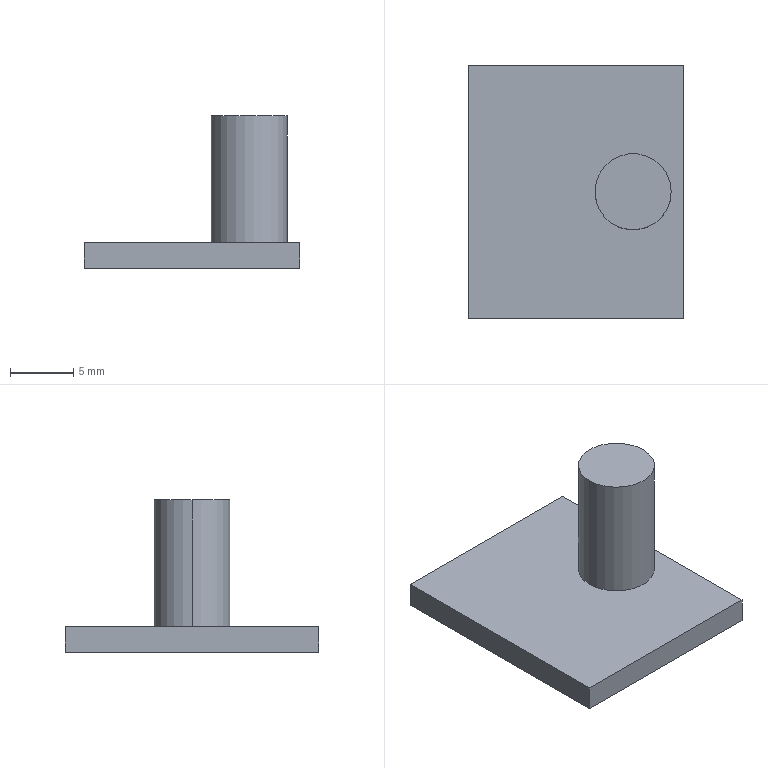Part | SolidWorks | features FlatPattern 1, ICE 1, SMBaseFlange 1, SheetMetal 1 | 1 solid | 9 faces | box 17 x 20 x 12 mm | volume 962.743 mm3 | plane 7 | cylinder 2 | commonest cylinder face diameters 6 x2
STEP:
#1=CARTESIAN_POINT('',(7.5,0.,10.));
#2=VERTEX_POINT('',#1);
#3=CARTESIAN_POINT('',(1.5,0.,10.));
#4=VERTEX_POINT('',#3);
#5=CARTESIAN_POINT('',(4.5,0.,10.));
#6=DIRECTION('',(0.,0.,1.));
#7=DIRECTION('',(1.,0.,0.));
#8=AXIS2_PLACEMENT_3D('',#5,#6,#7);
#9=CIRCLE('',#8,3.);
#10=EDGE_CURVE('',#2,#4,#9,.T.);
#11=ORIENTED_EDGE('',*,*,#10,.F.);
#12=CARTESIAN_POINT('',(7.5,0.,0.));
#13=VERTEX_POINT('',#12);
#14=CARTESIAN_POINT('',(7.5,0.,10.));
#15=DIRECTION('',(0.,0.,-1.));
#16=VECTOR('',#15,1000.);
#17=LINE('',#14,#16);
#18=EDGE_CURVE('',#2,#13,#17,.T.);
#19=ORIENTED_EDGE('',*,*,#18,.T.);
#20=CARTESIAN_POINT('',(1.5,0.,0.));
#21=VERTEX_POINT('',#20);
#22=CARTESIAN_POINT('',(4.5,0.,0.));
#23=DIRECTION('',(0.,0.,1.));
#24=DIRECTION('',(1.,0.,0.));
#25=AXIS2_PLACEMENT_3D('',#22,#23,#24);
#26=CIRCLE('',#25,3.);
#27=EDGE_CURVE('',#13,#21,#26,.T.);
#28=ORIENTED_EDGE('',*,*,#27,.T.);
#29=CARTESIAN_POINT('',(1.5,0.,10.));
#30=DIRECTION('',(0.,0.,-1.));
#31=VECTOR('',#30,1000.);
#32=LINE('',#29,#31);
#33=EDGE_CURVE('',#4,#21,#32,.T.);
#34=ORIENTED_EDGE('',*,*,#33,.F.);
#35=EDGE_LOOP('',(#11,#19,#28,#34));
#36=FACE_OUTER_BOUND('',#35,.T.);
#37=CARTESIAN_POINT('',(4.5,0.,10.));
#38=DIRECTION('',(0.,0.,-1.));
#39=DIRECTION('',(-1.,0.,0.));
#40=AXIS2_PLACEMENT_3D('',#37,#38,#39);
#41=CYLINDRICAL_SURFACE('',#40,3.);
#42=ADVANCED_FACE('',(#36),#41,.T.);
#43=CARTESIAN_POINT('',(8.5,-10.,0.));
#44=VERTEX_POINT('',#43);
#45=CARTESIAN_POINT('',(8.5,10.,0.));
#46=VERTEX_POINT('',#45);
#47=CARTESIAN_POINT('',(8.5,10.,0.));
#48=DIRECTION('',(0.,1.,0.));
#49=VECTOR('',#48,1000.);
#50=LINE('',#47,#49);
#51=EDGE_CURVE('',#44,#46,#50,.T.);
#52=ORIENTED_EDGE('',*,*,#51,.T.);
#53=CARTESIAN_POINT('',(-8.5,10.,0.));
#54=VERTEX_POINT('',#53);
#55=CARTESIAN_POINT('',(-8.5,10.,0.));
#56=DIRECTION('',(-1.,0.,0.));
#57=VECTOR('',#56,1000.);
#58=LINE('',#55,#57);
#59=EDGE_CURVE('',#46,#54,#58,.T.);
#60=ORIENTED_EDGE('',*,*,#59,.T.);
#61=CARTESIAN_POINT('',(-8.5,-10.,0.));
#62=VERTEX_POINT('',#61);
#63=CARTESIAN_POINT('',(-8.5,10.,0.));
#64=DIRECTION('',(0.,-1.,0.));
#65=VECTOR('',#64,1000.);
#66=LINE('',#63,#65);
#67=EDGE_CURVE('',#54,#62,#66,.T.);
#68=ORIENTED_EDGE('',*,*,#67,.T.);
#69=CARTESIAN_POINT('',(-8.5,-10.,0.));
#70=DIRECTION('',(1.,0.,0.));
#71=VECTOR('',#70,1000.);
#72=LINE('',#69,#71);
#73=EDGE_CURVE('',#62,#44,#72,.T.);
#74=ORIENTED_EDGE('',*,*,#73,.T.);
#75=EDGE_LOOP('',(#52,#60,#68,#74));
#76=FACE_OUTER_BOUND('',#75,.T.);
#77=CARTESIAN_POINT('',(4.5,0.,0.));
#78=DIRECTION('',(0.,0.,1.));
#79=DIRECTION('',(1.,0.,0.));
#80=AXIS2_PLACEMENT_3D('',#77,#78,#79);
#81=CIRCLE('',#80,3.);
#82=EDGE_CURVE('',#21,#13,#81,.T.);
#83=ORIENTED_EDGE('',*,*,#82,.F.);
#84=ORIENTED_EDGE('',*,*,#27,.F.);
#85=EDGE_LOOP('',(#83,#84));
#86=FACE_BOUND('',#85,.T.);
#87=CARTESIAN_POINT('',(0.,0.,0.));
#88=DIRECTION('',(0.,0.,1.));
#89=DIRECTION('',(1.,0.,0.));
#90=AXIS2_PLACEMENT_3D('',#87,#88,#89);
#91=PLANE('',#90);
#92=ADVANCED_FACE('',(#76,#86),#91,.T.);
#93=ORIENTED_EDGE('',*,*,#51,.F.);
#94=CARTESIAN_POINT('',(8.5,-10.,-2.));
#95=VERTEX_POINT('',#94);
#96=CARTESIAN_POINT('',(8.5,-10.,-2.));
#97=DIRECTION('',(0.,0.,1.));
#98=VECTOR('',#97,1000.);
#99=LINE('',#96,#98);
#100=EDGE_CURVE('',#95,#44,#99,.T.);
#101=ORIENTED_EDGE('',*,*,#100,.F.);
#102=CARTESIAN_POINT('',(8.5,10.,-2.));
#103=VERTEX_POINT('',#102);
#104=CARTESIAN_POINT('',(8.5,10.,-2.));
#105=DIRECTION('',(0.,1.,0.));
#106=VECTOR('',#105,1000.);
#107=LINE('',#104,#106);
#108=EDGE_CURVE('',#95,#103,#107,.T.);
#109=ORIENTED_EDGE('',*,*,#108,.T.);
#110=CARTESIAN_POINT('',(8.5,10.,-2.));
#111=DIRECTION('',(0.,0.,1.));
#112=VECTOR('',#111,1000.);
#113=LINE('',#110,#112);
#114=EDGE_CURVE('',#103,#46,#113,.T.);
#115=ORIENTED_EDGE('',*,*,#114,.T.);
#116=EDGE_LOOP('',(#93,#101,#109,#115));
#117=FACE_OUTER_BOUND('',#116,.T.);
#118=CARTESIAN_POINT('',(8.5,10.,-2.));
#119=DIRECTION('',(1.,0.,0.));
#120=DIRECTION('',(0.,1.,0.));
#121=AXIS2_PLACEMENT_3D('',#118,#119,#120);
#122=PLANE('',#121);
#123=ADVANCED_FACE('',(#117),#122,.T.);
#124=ORIENTED_EDGE('',*,*,#73,.F.);
#125=CARTESIAN_POINT('',(-8.5,-10.,-2.));
#126=VERTEX_POINT('',#125);
#127=CARTESIAN_POINT('',(-8.5,-10.,-2.));
#128=DIRECTION('',(0.,0.,1.));
#129=VECTOR('',#128,1000.);
#130=LINE('',#127,#129);
#131=EDGE_CURVE('',#126,#62,#130,.T.);
#132=ORIENTED_EDGE('',*,*,#131,.F.);
#133=CARTESIAN_POINT('',(-8.5,-10.,-2.));
#134=DIRECTION('',(1.,0.,0.));
#135=VECTOR('',#134,1000.);
#136=LINE('',#133,#135);
#137=EDGE_CURVE('',#126,#95,#136,.T.);
#138=ORIENTED_EDGE('',*,*,#137,.T.);
#139=ORIENTED_EDGE('',*,*,#100,.T.);
#140=EDGE_LOOP('',(#124,#132,#138,#139));
#141=FACE_OUTER_BOUND('',#140,.T.);
#142=CARTESIAN_POINT('',(-8.5,-10.,-2.));
#143=DIRECTION('',(0.,-1.,0.));
#144=DIRECTION('',(0.,0.,-1.));
#145=AXIS2_PLACEMENT_3D('',#142,#143,#144);
#146=PLANE('',#145);
#147=ADVANCED_FACE('',(#141),#146,.T.);
#148=ORIENTED_EDGE('',*,*,#67,.F.);
#149=CARTESIAN_POINT('',(-8.5,10.,-2.));
#150=VERTEX_POINT('',#149);
#151=CARTESIAN_POINT('',(-8.5,10.,-2.));
#152=DIRECTION('',(0.,0.,1.));
#153=VECTOR('',#152,1000.);
#154=LINE('',#151,#153);
#155=EDGE_CURVE('',#150,#54,#154,.T.);
#156=ORIENTED_EDGE('',*,*,#155,.F.);
#157=CARTESIAN_POINT('',(-8.5,10.,-2.));
#158=DIRECTION('',(0.,-1.,0.));
#159=VECTOR('',#158,1000.);
#160=LINE('',#157,#159);
#161=EDGE_CURVE('',#150,#126,#160,.T.);
#162=ORIENTED_EDGE('',*,*,#161,.T.);
#163=ORIENTED_EDGE('',*,*,#131,.T.);
#164=EDGE_LOOP('',(#148,#156,#162,#163));
#165=FACE_OUTER_BOUND('',#164,.T.);
#166=CARTESIAN_POINT('',(-8.5,10.,-2.));
#167=DIRECTION('',(-1.,0.,0.));
#168=DIRECTION('',(0.,-1.,0.));
#169=AXIS2_PLACEMENT_3D('',#166,#167,#168);
#170=PLANE('',#169);
#171=ADVANCED_FACE('',(#165),#170,.T.);
#172=ORIENTED_EDGE('',*,*,#59,.F.);
#173=ORIENTED_EDGE('',*,*,#114,.F.);
#174=CARTESIAN_POINT('',(-8.5,10.,-2.));
#175=DIRECTION('',(-1.,0.,0.));
#176=VECTOR('',#175,1000.);
#177=LINE('',#174,#176);
#178=EDGE_CURVE('',#103,#150,#177,.T.);
#179=ORIENTED_EDGE('',*,*,#178,.T.);
#180=ORIENTED_EDGE('',*,*,#155,.T.);
#181=EDGE_LOOP('',(#172,#173,#179,#180));
#182=FACE_OUTER_BOUND('',#181,.T.);
#183=CARTESIAN_POINT('',(-8.5,10.,-2.));
#184=DIRECTION('',(0.,1.,0.));
#185=DIRECTION('',(0.,0.,1.));
#186=AXIS2_PLACEMENT_3D('',#183,#184,#185);
#187=PLANE('',#186);
#188=ADVANCED_FACE('',(#182),#187,.T.);
#189=ORIENTED_EDGE('',*,*,#108,.F.);
#190=ORIENTED_EDGE('',*,*,#137,.F.);
#191=ORIENTED_EDGE('',*,*,#161,.F.);
#192=ORIENTED_EDGE('',*,*,#178,.F.);
#193=EDGE_LOOP('',(#189,#190,#191,#192));
#194=FACE_OUTER_BOUND('',#193,.T.);
#195=CARTESIAN_POINT('',(0.,0.,-2.));
#196=DIRECTION('',(0.,0.,1.));
#197=DIRECTION('',(1.,0.,0.));
#198=AXIS2_PLACEMENT_3D('',#195,#196,#197);
#199=PLANE('',#198);
#200=ADVANCED_FACE('',(#194),#199,.F.);
#201=ORIENTED_EDGE('',*,*,#18,.F.);
#202=CARTESIAN_POINT('',(4.5,0.,10.));
#203=DIRECTION('',(0.,0.,1.));
#204=DIRECTION('',(1.,0.,0.));
#205=AXIS2_PLACEMENT_3D('',#202,#203,#204);
#206=CIRCLE('',#205,3.);
#207=EDGE_CURVE('',#4,#2,#206,.T.);
#208=ORIENTED_EDGE('',*,*,#207,.F.);
#209=ORIENTED_EDGE('',*,*,#33,.T.);
#210=ORIENTED_EDGE('',*,*,#82,.T.);
#211=EDGE_LOOP('',(#201,#208,#209,#210));
#212=FACE_OUTER_BOUND('',#211,.T.);
#213=CARTESIAN_POINT('',(4.5,0.,10.));
#214=DIRECTION('',(0.,0.,-1.));
#215=DIRECTION('',(-1.,0.,0.));
#216=AXIS2_PLACEMENT_3D('',#213,#214,#215);
#217=CYLINDRICAL_SURFACE('',#216,3.);
#218=ADVANCED_FACE('',(#212),#217,.T.);
#219=ORIENTED_EDGE('',*,*,#207,.T.);
#220=ORIENTED_EDGE('',*,*,#10,.T.);
#221=EDGE_LOOP('',(#219,#220));
#222=FACE_OUTER_BOUND('',#221,.T.);
#223=CARTESIAN_POINT('',(4.5,0.,10.));
#224=DIRECTION('',(0.,0.,1.));
#225=DIRECTION('',(1.,0.,0.));
#226=AXIS2_PLACEMENT_3D('',#223,#224,#225);
#227=PLANE('',#226);
#228=ADVANCED_FACE('',(#222),#227,.T.);
#229=CLOSED_SHELL('',(#42,#92,#123,#147,#171,#188,#200,#218,#228));
#230=MANIFOLD_SOLID_BREP('',#229);
#231=CARTESIAN_POINT('',(0.,0.,0.));
#232=DIRECTION('',(0.,0.,1.));
#233=DIRECTION('',(1.,0.,0.));
#234=AXIS2_PLACEMENT_3D('',#231,#232,#233);
#235=(LENGTH_UNIT()NAMED_UNIT(*)SI_UNIT(.MILLI.,.METRE.));
#236=UNCERTAINTY_MEASURE_WITH_UNIT(LENGTH_MEASURE(0.00001),#235,'','');
#237=(NAMED_UNIT(*)PLANE_ANGLE_UNIT()SI_UNIT($,.RADIAN.));
#238=(NAMED_UNIT(*)SI_UNIT($,.STERADIAN.)SOLID_ANGLE_UNIT());
#239=(GEOMETRIC_REPRESENTATION_CONTEXT(3)GLOBAL_UNCERTAINTY_ASSIGNED_CONTEXT((#236))GLOBAL_UNIT_ASSIGNED_CONTEXT((#235,#237,#238))REPRESENTATION_CONTEXT('',''));
#240=ADVANCED_BREP_SHAPE_REPRESENTATION('',(#230,#234),#239);